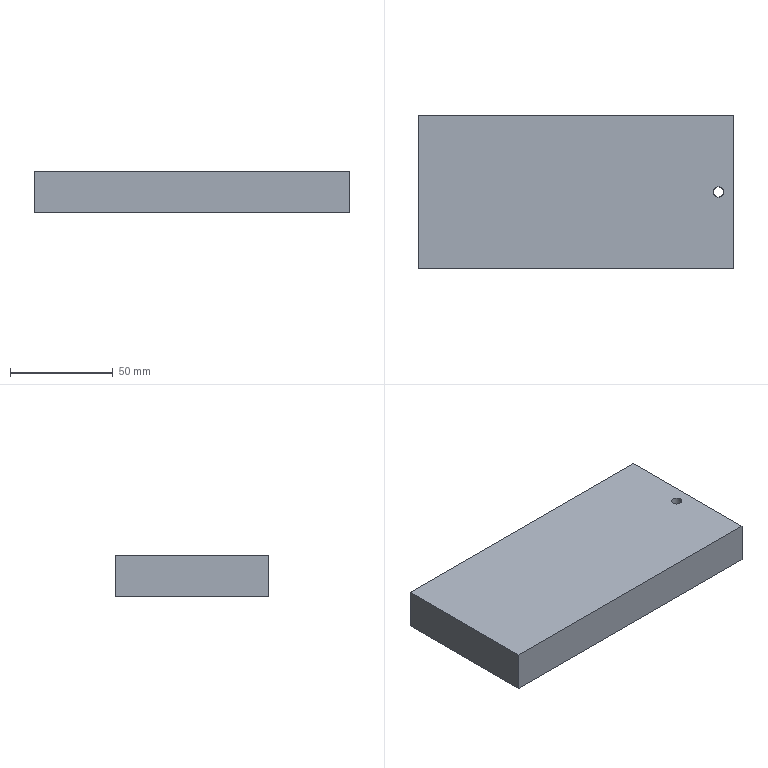Part | STEP file | Positioning_id762_x_t | 1 solid | 13 faces | box 154.003 x 75 x 20 mm | volume 229388 mm3 | plane 7 | cylinder 6 | commonest cylinder face diameters 5 x4 10 x2